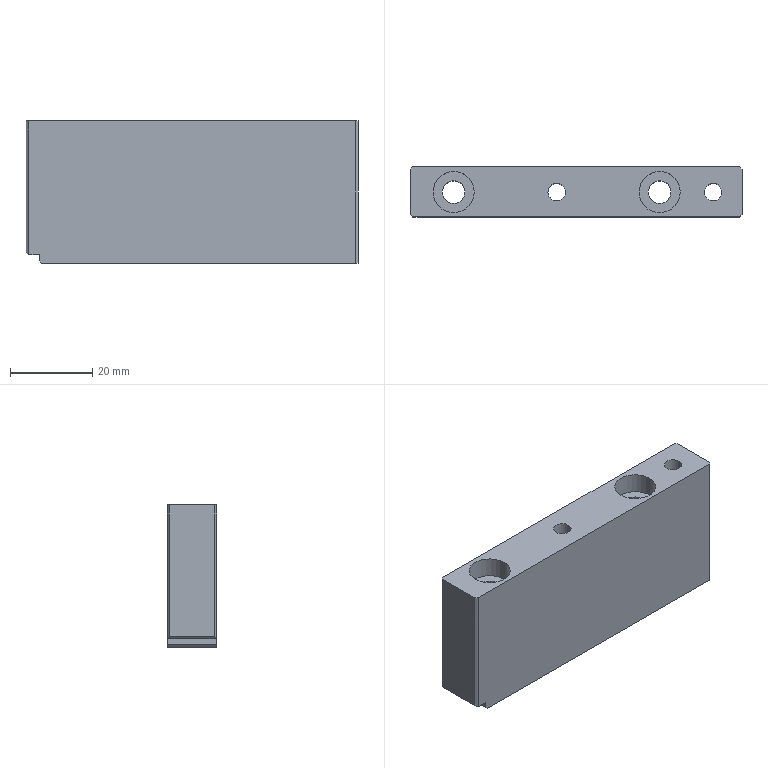Part | STEP file | side block 2-2 | 1 solid | 28 faces | box 80.6 x 12.1 x 34.5 mm | volume 30402 mm3 | plane 16 | cylinder 12 | commonest cylinder face diameters 4.2 x4 5.5 x4 10 x4